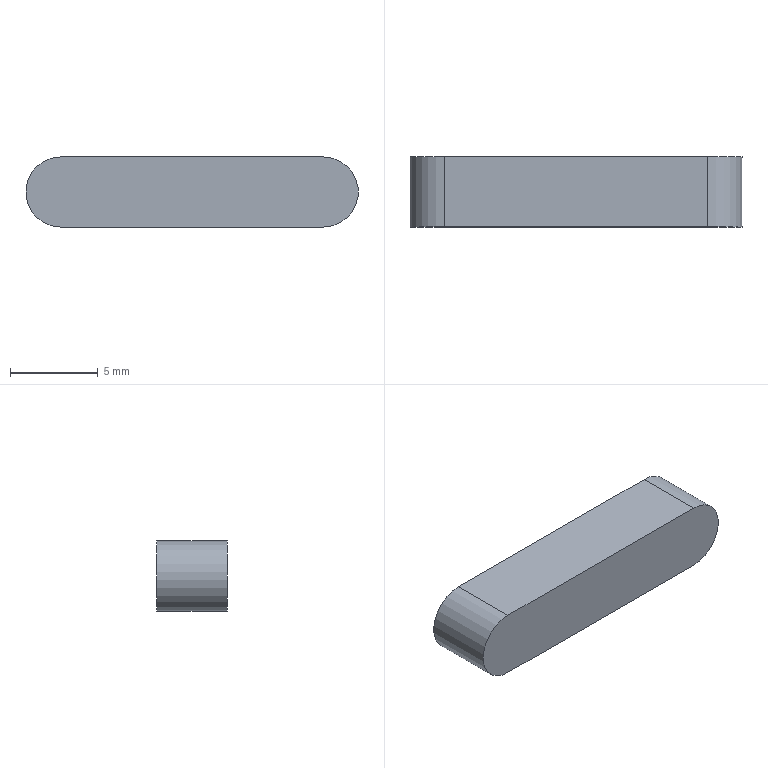Part | STEP file | PN_0038 (4x4x15) | 1 solid | 6 faces | box 19 x 4 x 4 mm | volume 290.265 mm3 | plane 4 | cylinder 2 | commonest cylinder face diameters 4 x2
STEP:
#1=CARTESIAN_POINT('',(0.,0.,0.));
#2=DIRECTION('',(0.,0.,1.));
#3=DIRECTION('',(1.,0.,0.));
#4=AXIS2_PLACEMENT_3D('',#1,#2,#3);
#5=CARTESIAN_POINT('',(-7.5,0.,-2.));
#6=VERTEX_POINT('',#5);
#7=CARTESIAN_POINT('',(-7.5,0.,2.));
#8=VERTEX_POINT('',#7);
#9=CARTESIAN_POINT('',(-7.5,0.,0.));
#10=DIRECTION('',(0.,1.,0.));
#11=DIRECTION('',(0.,0.,1.));
#12=AXIS2_PLACEMENT_3D('',#9,#10,#11);
#13=CIRCLE('',#12,2.);
#14=CARTESIAN_POINT('',(-7.5,4.,0.));
#15=DIRECTION('',(0.,-1.,0.));
#16=DIRECTION('',(0.,0.,-1.));
#17=AXIS2_PLACEMENT_3D('',#14,#15,#16);
#18=CYLINDRICAL_SURFACE('',#17,2.);
#19=CARTESIAN_POINT('',(9.425,4.));
#20=DIRECTION('',(-1.,0.));
#21=VECTOR('',#20,1.);
#22=LINE('',#19,#21);
#23=(GEOMETRIC_REPRESENTATION_CONTEXT(2)PARAMETRIC_REPRESENTATION_CONTEXT()REPRESENTATION_CONTEXT('',''));
#24=DEFINITIONAL_REPRESENTATION('',(#22),#23);
#25=PCURVE('',#18,#24);
#26=CARTESIAN_POINT('',(-7.5,0.,0.));
#27=DIRECTION('',(0.,1.,0.));
#28=DIRECTION('',(0.,0.,1.));
#29=AXIS2_PLACEMENT_3D('',#26,#27,#28);
#30=PLANE('',#29);
#31=CARTESIAN_POINT('',(0.,0.));
#32=DIRECTION('',(1.,0.));
#33=AXIS2_PLACEMENT_2D('',#31,#32);
#34=CIRCLE('',#33,2.);
#35=(GEOMETRIC_REPRESENTATION_CONTEXT(2)PARAMETRIC_REPRESENTATION_CONTEXT()REPRESENTATION_CONTEXT('',''));
#36=DEFINITIONAL_REPRESENTATION('',(#34),#35);
#37=PCURVE('',#30,#36);
#38=SURFACE_CURVE('',#13,(#25,#37),.PCURVE_S1.);
#39=EDGE_CURVE('',#6,#8,#38,.T.);
#40=ORIENTED_EDGE('',*,*,#39,.T.);
#41=CARTESIAN_POINT('',(-7.5,4.,2.));
#42=VERTEX_POINT('',#41);
#43=CARTESIAN_POINT('',(-7.5,4.,2.));
#44=DIRECTION('',(0.,-1.,0.));
#45=VECTOR('',#44,1.);
#46=LINE('',#43,#45);
#47=CARTESIAN_POINT('',(3.142,0.));
#48=DIRECTION('',(0.,1.));
#49=VECTOR('',#48,1.);
#50=LINE('',#47,#49);
#51=(GEOMETRIC_REPRESENTATION_CONTEXT(2)PARAMETRIC_REPRESENTATION_CONTEXT()REPRESENTATION_CONTEXT('',''));
#52=DEFINITIONAL_REPRESENTATION('',(#50),#51);
#53=PCURVE('',#18,#52);
#54=CARTESIAN_POINT('',(-7.5,4.,2.));
#55=DIRECTION('',(0.,0.,-1.));
#56=DIRECTION('',(-1.,0.,0.));
#57=AXIS2_PLACEMENT_3D('',#54,#55,#56);
#58=PLANE('',#57);
#59=CARTESIAN_POINT('',(0.,0.));
#60=DIRECTION('',(0.,-1.));
#61=VECTOR('',#60,1.);
#62=LINE('',#59,#61);
#63=(GEOMETRIC_REPRESENTATION_CONTEXT(2)PARAMETRIC_REPRESENTATION_CONTEXT()REPRESENTATION_CONTEXT('',''));
#64=DEFINITIONAL_REPRESENTATION('',(#62),#63);
#65=PCURVE('',#58,#64);
#66=SURFACE_CURVE('',#46,(#53,#65),.PCURVE_S1.);
#67=EDGE_CURVE('',#42,#8,#66,.T.);
#68=ORIENTED_EDGE('',*,*,#67,.F.);
#69=CARTESIAN_POINT('',(-7.5,4.,-2.));
#70=VERTEX_POINT('',#69);
#71=CARTESIAN_POINT('',(-7.5,4.,0.));
#72=DIRECTION('',(0.,1.,0.));
#73=DIRECTION('',(0.,0.,1.));
#74=AXIS2_PLACEMENT_3D('',#71,#72,#73);
#75=CIRCLE('',#74,2.);
#76=CARTESIAN_POINT('',(9.425,0.));
#77=DIRECTION('',(-1.,0.));
#78=VECTOR('',#77,1.);
#79=LINE('',#76,#78);
#80=(GEOMETRIC_REPRESENTATION_CONTEXT(2)PARAMETRIC_REPRESENTATION_CONTEXT()REPRESENTATION_CONTEXT('',''));
#81=DEFINITIONAL_REPRESENTATION('',(#79),#80);
#82=PCURVE('',#18,#81);
#83=CARTESIAN_POINT('',(-7.5,4.,0.));
#84=DIRECTION('',(0.,1.,0.));
#85=DIRECTION('',(0.,0.,1.));
#86=AXIS2_PLACEMENT_3D('',#83,#84,#85);
#87=PLANE('',#86);
#88=CARTESIAN_POINT('',(0.,0.));
#89=DIRECTION('',(1.,0.));
#90=AXIS2_PLACEMENT_2D('',#88,#89);
#91=CIRCLE('',#90,2.);
#92=(GEOMETRIC_REPRESENTATION_CONTEXT(2)PARAMETRIC_REPRESENTATION_CONTEXT()REPRESENTATION_CONTEXT('',''));
#93=DEFINITIONAL_REPRESENTATION('',(#91),#92);
#94=PCURVE('',#87,#93);
#95=SURFACE_CURVE('',#75,(#82,#94),.PCURVE_S1.);
#96=EDGE_CURVE('',#70,#42,#95,.T.);
#97=ORIENTED_EDGE('',*,*,#96,.F.);
#98=CARTESIAN_POINT('',(-7.5,4.,-2.));
#99=DIRECTION('',(0.,-1.,0.));
#100=VECTOR('',#99,1.);
#101=LINE('',#98,#100);
#102=CARTESIAN_POINT('',(6.283,0.));
#103=DIRECTION('',(0.,1.));
#104=VECTOR('',#103,1.);
#105=LINE('',#102,#104);
#106=(GEOMETRIC_REPRESENTATION_CONTEXT(2)PARAMETRIC_REPRESENTATION_CONTEXT()REPRESENTATION_CONTEXT('',''));
#107=DEFINITIONAL_REPRESENTATION('',(#105),#106);
#108=PCURVE('',#18,#107);
#109=CARTESIAN_POINT('',(-7.5,4.,-2.));
#110=DIRECTION('',(0.,0.,1.));
#111=DIRECTION('',(1.,0.,0.));
#112=AXIS2_PLACEMENT_3D('',#109,#110,#111);
#113=PLANE('',#112);
#114=CARTESIAN_POINT('',(0.,0.));
#115=DIRECTION('',(0.,-1.));
#116=VECTOR('',#115,1.);
#117=LINE('',#114,#116);
#118=(GEOMETRIC_REPRESENTATION_CONTEXT(2)PARAMETRIC_REPRESENTATION_CONTEXT()REPRESENTATION_CONTEXT('',''));
#119=DEFINITIONAL_REPRESENTATION('',(#117),#118);
#120=PCURVE('',#113,#119);
#121=SURFACE_CURVE('',#101,(#108,#120),.PCURVE_S1.);
#122=EDGE_CURVE('',#70,#6,#121,.T.);
#123=ORIENTED_EDGE('',*,*,#122,.T.);
#124=EDGE_LOOP('',(#40,#68,#97,#123));
#125=FACE_BOUND('',#124,.T.);
#126=ADVANCED_FACE('',(#125),#18,.T.);
#127=CARTESIAN_POINT('',(7.5,0.,2.));
#128=VERTEX_POINT('',#127);
#129=CARTESIAN_POINT('',(-7.5,0.,2.));
#130=DIRECTION('',(1.,0.,0.));
#131=VECTOR('',#130,1.);
#132=LINE('',#129,#131);
#133=CARTESIAN_POINT('',(0.,-4.));
#134=DIRECTION('',(-1.,0.));
#135=VECTOR('',#134,1.);
#136=LINE('',#133,#135);
#137=(GEOMETRIC_REPRESENTATION_CONTEXT(2)PARAMETRIC_REPRESENTATION_CONTEXT()REPRESENTATION_CONTEXT('',''));
#138=DEFINITIONAL_REPRESENTATION('',(#136),#137);
#139=PCURVE('',#58,#138);
#140=CARTESIAN_POINT('',(2.,0.));
#141=DIRECTION('',(0.,1.));
#142=VECTOR('',#141,1.);
#143=LINE('',#140,#142);
#144=(GEOMETRIC_REPRESENTATION_CONTEXT(2)PARAMETRIC_REPRESENTATION_CONTEXT()REPRESENTATION_CONTEXT('',''));
#145=DEFINITIONAL_REPRESENTATION('',(#143),#144);
#146=PCURVE('',#30,#145);
#147=SURFACE_CURVE('',#132,(#139,#146),.PCURVE_S1.);
#148=EDGE_CURVE('',#8,#128,#147,.T.);
#149=ORIENTED_EDGE('',*,*,#148,.T.);
#150=CARTESIAN_POINT('',(7.5,4.,2.));
#151=VERTEX_POINT('',#150);
#152=CARTESIAN_POINT('',(7.5,4.,2.));
#153=DIRECTION('',(0.,-1.,0.));
#154=VECTOR('',#153,1.);
#155=LINE('',#152,#154);
#156=CARTESIAN_POINT('',(-15.,0.));
#157=DIRECTION('',(0.,-1.));
#158=VECTOR('',#157,1.);
#159=LINE('',#156,#158);
#160=(GEOMETRIC_REPRESENTATION_CONTEXT(2)PARAMETRIC_REPRESENTATION_CONTEXT()REPRESENTATION_CONTEXT('',''));
#161=DEFINITIONAL_REPRESENTATION('',(#159),#160);
#162=PCURVE('',#58,#161);
#163=CARTESIAN_POINT('',(7.5,4.,0.));
#164=DIRECTION('',(0.,-1.,0.));
#165=DIRECTION('',(0.,0.,-1.));
#166=AXIS2_PLACEMENT_3D('',#163,#164,#165);
#167=CYLINDRICAL_SURFACE('',#166,2.);
#168=CARTESIAN_POINT('',(3.142,0.));
#169=DIRECTION('',(0.,1.));
#170=VECTOR('',#169,1.);
#171=LINE('',#168,#170);
#172=(GEOMETRIC_REPRESENTATION_CONTEXT(2)PARAMETRIC_REPRESENTATION_CONTEXT()REPRESENTATION_CONTEXT('',''));
#173=DEFINITIONAL_REPRESENTATION('',(#171),#172);
#174=PCURVE('',#167,#173);
#175=SURFACE_CURVE('',#155,(#162,#174),.PCURVE_S1.);
#176=EDGE_CURVE('',#151,#128,#175,.T.);
#177=ORIENTED_EDGE('',*,*,#176,.F.);
#178=CARTESIAN_POINT('',(-7.5,4.,2.));
#179=DIRECTION('',(1.,0.,0.));
#180=VECTOR('',#179,1.);
#181=LINE('',#178,#180);
#182=CARTESIAN_POINT('',(0.,0.));
#183=DIRECTION('',(-1.,0.));
#184=VECTOR('',#183,1.);
#185=LINE('',#182,#184);
#186=(GEOMETRIC_REPRESENTATION_CONTEXT(2)PARAMETRIC_REPRESENTATION_CONTEXT()REPRESENTATION_CONTEXT('',''));
#187=DEFINITIONAL_REPRESENTATION('',(#185),#186);
#188=PCURVE('',#58,#187);
#189=CARTESIAN_POINT('',(2.,0.));
#190=DIRECTION('',(0.,1.));
#191=VECTOR('',#190,1.);
#192=LINE('',#189,#191);
#193=(GEOMETRIC_REPRESENTATION_CONTEXT(2)PARAMETRIC_REPRESENTATION_CONTEXT()REPRESENTATION_CONTEXT('',''));
#194=DEFINITIONAL_REPRESENTATION('',(#192),#193);
#195=PCURVE('',#87,#194);
#196=SURFACE_CURVE('',#181,(#188,#195),.PCURVE_S1.);
#197=EDGE_CURVE('',#42,#151,#196,.T.);
#198=ORIENTED_EDGE('',*,*,#197,.F.);
#199=ORIENTED_EDGE('',*,*,#67,.T.);
#200=EDGE_LOOP('',(#149,#177,#198,#199));
#201=FACE_BOUND('',#200,.T.);
#202=ADVANCED_FACE('',(#201),#58,.F.);
#203=CARTESIAN_POINT('',(7.5,0.,-2.));
#204=VERTEX_POINT('',#203);
#205=CARTESIAN_POINT('',(7.5,0.,0.));
#206=DIRECTION('',(0.,1.,0.));
#207=DIRECTION('',(0.,0.,1.));
#208=AXIS2_PLACEMENT_3D('',#205,#206,#207);
#209=CIRCLE('',#208,2.);
#210=CARTESIAN_POINT('',(3.142,4.));
#211=DIRECTION('',(-1.,0.));
#212=VECTOR('',#211,1.);
#213=LINE('',#210,#212);
#214=(GEOMETRIC_REPRESENTATION_CONTEXT(2)PARAMETRIC_REPRESENTATION_CONTEXT()REPRESENTATION_CONTEXT('',''));
#215=DEFINITIONAL_REPRESENTATION('',(#213),#214);
#216=PCURVE('',#167,#215);
#217=CARTESIAN_POINT('',(0.,15.));
#218=DIRECTION('',(1.,0.));
#219=AXIS2_PLACEMENT_2D('',#217,#218);
#220=CIRCLE('',#219,2.);
#221=(GEOMETRIC_REPRESENTATION_CONTEXT(2)PARAMETRIC_REPRESENTATION_CONTEXT()REPRESENTATION_CONTEXT('',''));
#222=DEFINITIONAL_REPRESENTATION('',(#220),#221);
#223=PCURVE('',#30,#222);
#224=SURFACE_CURVE('',#209,(#216,#223),.PCURVE_S1.);
#225=EDGE_CURVE('',#128,#204,#224,.T.);
#226=ORIENTED_EDGE('',*,*,#225,.T.);
#227=CARTESIAN_POINT('',(7.5,4.,-2.));
#228=VERTEX_POINT('',#227);
#229=CARTESIAN_POINT('',(7.5,4.,-2.));
#230=DIRECTION('',(0.,-1.,0.));
#231=VECTOR('',#230,1.);
#232=LINE('',#229,#231);
#233=CARTESIAN_POINT('',(0.,0.));
#234=DIRECTION('',(0.,1.));
#235=VECTOR('',#234,1.);
#236=LINE('',#233,#235);
#237=(GEOMETRIC_REPRESENTATION_CONTEXT(2)PARAMETRIC_REPRESENTATION_CONTEXT()REPRESENTATION_CONTEXT('',''));
#238=DEFINITIONAL_REPRESENTATION('',(#236),#237);
#239=PCURVE('',#167,#238);
#240=CARTESIAN_POINT('',(15.,0.));
#241=DIRECTION('',(0.,-1.));
#242=VECTOR('',#241,1.);
#243=LINE('',#240,#242);
#244=(GEOMETRIC_REPRESENTATION_CONTEXT(2)PARAMETRIC_REPRESENTATION_CONTEXT()REPRESENTATION_CONTEXT('',''));
#245=DEFINITIONAL_REPRESENTATION('',(#243),#244);
#246=PCURVE('',#113,#245);
#247=SURFACE_CURVE('',#232,(#239,#246),.PCURVE_S1.);
#248=EDGE_CURVE('',#228,#204,#247,.T.);
#249=ORIENTED_EDGE('',*,*,#248,.F.);
#250=CARTESIAN_POINT('',(7.5,4.,0.));
#251=DIRECTION('',(0.,1.,0.));
#252=DIRECTION('',(0.,0.,1.));
#253=AXIS2_PLACEMENT_3D('',#250,#251,#252);
#254=CIRCLE('',#253,2.);
#255=CARTESIAN_POINT('',(3.142,0.));
#256=DIRECTION('',(-1.,0.));
#257=VECTOR('',#256,1.);
#258=LINE('',#255,#257);
#259=(GEOMETRIC_REPRESENTATION_CONTEXT(2)PARAMETRIC_REPRESENTATION_CONTEXT()REPRESENTATION_CONTEXT('',''));
#260=DEFINITIONAL_REPRESENTATION('',(#258),#259);
#261=PCURVE('',#167,#260);
#262=CARTESIAN_POINT('',(0.,15.));
#263=DIRECTION('',(1.,0.));
#264=AXIS2_PLACEMENT_2D('',#262,#263);
#265=CIRCLE('',#264,2.);
#266=(GEOMETRIC_REPRESENTATION_CONTEXT(2)PARAMETRIC_REPRESENTATION_CONTEXT()REPRESENTATION_CONTEXT('',''));
#267=DEFINITIONAL_REPRESENTATION('',(#265),#266);
#268=PCURVE('',#87,#267);
#269=SURFACE_CURVE('',#254,(#261,#268),.PCURVE_S1.);
#270=EDGE_CURVE('',#151,#228,#269,.T.);
#271=ORIENTED_EDGE('',*,*,#270,.F.);
#272=ORIENTED_EDGE('',*,*,#176,.T.);
#273=EDGE_LOOP('',(#226,#249,#271,#272));
#274=FACE_BOUND('',#273,.T.);
#275=ADVANCED_FACE('',(#274),#167,.T.);
#276=CARTESIAN_POINT('',(-7.5,0.,-2.));
#277=DIRECTION('',(-1.,0.,0.));
#278=VECTOR('',#277,1.);
#279=LINE('',#276,#278);
#280=CARTESIAN_POINT('',(0.,-4.));
#281=DIRECTION('',(-1.,0.));
#282=VECTOR('',#281,1.);
#283=LINE('',#280,#282);
#284=(GEOMETRIC_REPRESENTATION_CONTEXT(2)PARAMETRIC_REPRESENTATION_CONTEXT()REPRESENTATION_CONTEXT('',''));
#285=DEFINITIONAL_REPRESENTATION('',(#283),#284);
#286=PCURVE('',#113,#285);
#287=CARTESIAN_POINT('',(-2.,0.));
#288=DIRECTION('',(0.,-1.));
#289=VECTOR('',#288,1.);
#290=LINE('',#287,#289);
#291=(GEOMETRIC_REPRESENTATION_CONTEXT(2)PARAMETRIC_REPRESENTATION_CONTEXT()REPRESENTATION_CONTEXT('',''));
#292=DEFINITIONAL_REPRESENTATION('',(#290),#291);
#293=PCURVE('',#30,#292);
#294=SURFACE_CURVE('',#279,(#286,#293),.PCURVE_S1.);
#295=EDGE_CURVE('',#204,#6,#294,.T.);
#296=ORIENTED_EDGE('',*,*,#295,.T.);
#297=ORIENTED_EDGE('',*,*,#122,.F.);
#298=CARTESIAN_POINT('',(-7.5,4.,-2.));
#299=DIRECTION('',(-1.,0.,0.));
#300=VECTOR('',#299,1.);
#301=LINE('',#298,#300);
#302=CARTESIAN_POINT('',(0.,0.));
#303=DIRECTION('',(-1.,0.));
#304=VECTOR('',#303,1.);
#305=LINE('',#302,#304);
#306=(GEOMETRIC_REPRESENTATION_CONTEXT(2)PARAMETRIC_REPRESENTATION_CONTEXT()REPRESENTATION_CONTEXT('',''));
#307=DEFINITIONAL_REPRESENTATION('',(#305),#306);
#308=PCURVE('',#113,#307);
#309=CARTESIAN_POINT('',(-2.,0.));
#310=DIRECTION('',(0.,-1.));
#311=VECTOR('',#310,1.);
#312=LINE('',#309,#311);
#313=(GEOMETRIC_REPRESENTATION_CONTEXT(2)PARAMETRIC_REPRESENTATION_CONTEXT()REPRESENTATION_CONTEXT('',''));
#314=DEFINITIONAL_REPRESENTATION('',(#312),#313);
#315=PCURVE('',#87,#314);
#316=SURFACE_CURVE('',#301,(#308,#315),.PCURVE_S1.);
#317=EDGE_CURVE('',#228,#70,#316,.T.);
#318=ORIENTED_EDGE('',*,*,#317,.F.);
#319=ORIENTED_EDGE('',*,*,#248,.T.);
#320=EDGE_LOOP('',(#296,#297,#318,#319));
#321=FACE_BOUND('',#320,.T.);
#322=ADVANCED_FACE('',(#321),#113,.F.);
#323=ORIENTED_EDGE('',*,*,#96,.T.);
#324=ORIENTED_EDGE('',*,*,#197,.T.);
#325=ORIENTED_EDGE('',*,*,#270,.T.);
#326=ORIENTED_EDGE('',*,*,#317,.T.);
#327=EDGE_LOOP('',(#323,#324,#325,#326));
#328=FACE_BOUND('',#327,.T.);
#329=ADVANCED_FACE('',(#328),#87,.T.);
#330=ORIENTED_EDGE('',*,*,#39,.F.);
#331=ORIENTED_EDGE('',*,*,#295,.F.);
#332=ORIENTED_EDGE('',*,*,#225,.F.);
#333=ORIENTED_EDGE('',*,*,#148,.F.);
#334=EDGE_LOOP('',(#330,#331,#332,#333));
#335=FACE_BOUND('',#334,.T.);
#336=ADVANCED_FACE('',(#335),#30,.F.);
#337=CLOSED_SHELL('',(#126,#202,#275,#322,#329,#336));
#338=MANIFOLD_SOLID_BREP('',#337);
#339=(LENGTH_UNIT()NAMED_UNIT(*)SI_UNIT(.MILLI.,.METRE.));
#340=UNCERTAINTY_MEASURE_WITH_UNIT(LENGTH_MEASURE(0.0000001),#339,'','');
#341=(NAMED_UNIT(*)PLANE_ANGLE_UNIT()SI_UNIT($,.RADIAN.));
#342=(NAMED_UNIT(*)SI_UNIT($,.STERADIAN.)SOLID_ANGLE_UNIT());
#343=(GEOMETRIC_REPRESENTATION_CONTEXT(3)GLOBAL_UNCERTAINTY_ASSIGNED_CONTEXT((#340))GLOBAL_UNIT_ASSIGNED_CONTEXT((#339,#341,#342))REPRESENTATION_CONTEXT('',''));
#344=ADVANCED_BREP_SHAPE_REPRESENTATION('',(#4,#338),#343);